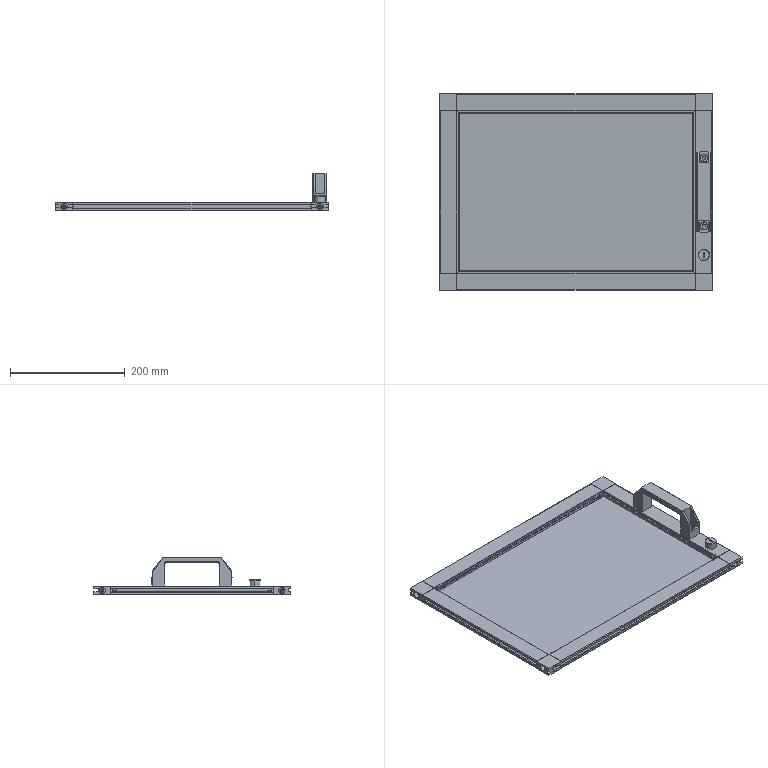Part | NX | features BREP 13 | 27 solids | 1017 faces | box 475 x 342 x 65 mm | volume 840442 mm3 | plane 626 | cylinder 275 | cone 64 | torus 44 | spline 4 | sphere 4 | commonest cylinder face diameters 1 x42 5 x39 2 x32 11 x32 0.4 x24 6 x18